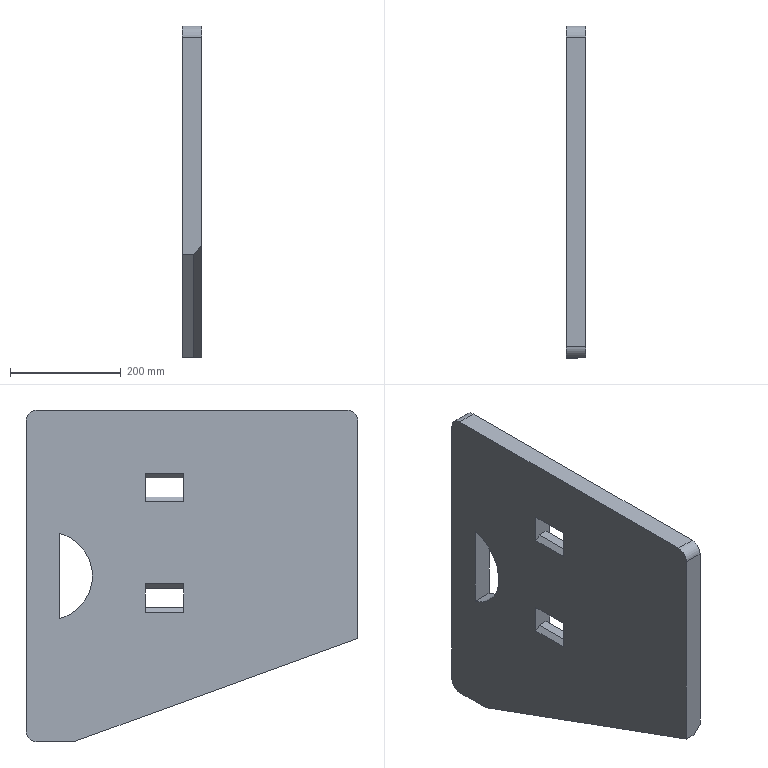Part | SolidWorks | features Chamfer 1, Extrusion 1, Fillet 1, ICE 1 | 1 solid | 29 faces | box 35 x 600 x 600 mm | volume 10412431 mm3 | plane 25 | cylinder 4 | commonest cylinder face diameters 40 x3 160 x1
STEP:
#1=CARTESIAN_POINT('',(17.5,15.,-366.));
#2=VERTEX_POINT('',#1);
#3=CARTESIAN_POINT('',(17.5,85.,-366.));
#4=VERTEX_POINT('',#3);
#5=CARTESIAN_POINT('',(17.5,15.,-366.));
#6=DIRECTION('',(0.,1.,0.));
#7=VECTOR('',#6,1000.);
#8=LINE('',#5,#7);
#9=EDGE_CURVE('',#2,#4,#8,.T.);
#10=ORIENTED_EDGE('',*,*,#9,.F.);
#11=CARTESIAN_POINT('',(17.5,15.,-314.));
#12=VERTEX_POINT('',#11);
#13=CARTESIAN_POINT('',(17.5,15.,-366.));
#14=DIRECTION('',(0.,0.,-1.));
#15=VECTOR('',#14,1000.);
#16=LINE('',#13,#15);
#17=EDGE_CURVE('',#12,#2,#16,.T.);
#18=ORIENTED_EDGE('',*,*,#17,.F.);
#19=CARTESIAN_POINT('',(17.5,85.,-314.));
#20=VERTEX_POINT('',#19);
#21=CARTESIAN_POINT('',(17.5,15.,-314.));
#22=DIRECTION('',(0.,1.,0.));
#23=VECTOR('',#22,1000.);
#24=LINE('',#21,#23);
#25=EDGE_CURVE('',#12,#20,#24,.T.);
#26=ORIENTED_EDGE('',*,*,#25,.T.);
#27=CARTESIAN_POINT('',(17.5,85.,-366.));
#28=DIRECTION('',(0.,0.,-1.));
#29=VECTOR('',#28,1000.);
#30=LINE('',#27,#29);
#31=EDGE_CURVE('',#20,#4,#30,.T.);
#32=ORIENTED_EDGE('',*,*,#31,.T.);
#33=EDGE_LOOP('',(#10,#18,#26,#32));
#34=FACE_BOUND('',#33,.T.);
#35=CARTESIAN_POINT('',(17.5,15.,-166.));
#36=VERTEX_POINT('',#35);
#37=CARTESIAN_POINT('',(17.5,85.,-166.));
#38=VERTEX_POINT('',#37);
#39=CARTESIAN_POINT('',(17.5,15.,-166.));
#40=DIRECTION('',(0.,1.,0.));
#41=VECTOR('',#40,1000.);
#42=LINE('',#39,#41);
#43=EDGE_CURVE('',#36,#38,#42,.T.);
#44=ORIENTED_EDGE('',*,*,#43,.F.);
#45=CARTESIAN_POINT('',(17.5,15.,-114.));
#46=VERTEX_POINT('',#45);
#47=CARTESIAN_POINT('',(17.5,15.,-114.));
#48=DIRECTION('',(0.,0.,-1.));
#49=VECTOR('',#48,1000.);
#50=LINE('',#47,#49);
#51=EDGE_CURVE('',#46,#36,#50,.T.);
#52=ORIENTED_EDGE('',*,*,#51,.F.);
#53=CARTESIAN_POINT('',(17.5,85.,-114.));
#54=VERTEX_POINT('',#53);
#55=CARTESIAN_POINT('',(17.5,15.,-114.));
#56=DIRECTION('',(0.,1.,0.));
#57=VECTOR('',#56,1000.);
#58=LINE('',#55,#57);
#59=EDGE_CURVE('',#46,#54,#58,.T.);
#60=ORIENTED_EDGE('',*,*,#59,.T.);
#61=CARTESIAN_POINT('',(17.5,85.,-114.));
#62=DIRECTION('',(0.,0.,-1.));
#63=VECTOR('',#62,1000.);
#64=LINE('',#61,#63);
#65=EDGE_CURVE('',#54,#38,#64,.T.);
#66=ORIENTED_EDGE('',*,*,#65,.T.);
#67=EDGE_LOOP('',(#44,#52,#60,#66));
#68=FACE_BOUND('',#67,.T.);
#69=CARTESIAN_POINT('',(17.5,-300.,-20.));
#70=VERTEX_POINT('',#69);
#71=CARTESIAN_POINT('',(17.5,-300.,-397.037));
#72=VERTEX_POINT('',#71);
#73=CARTESIAN_POINT('',(17.5,-300.,-413.));
#74=DIRECTION('',(0.,0.,-1.));
#75=VECTOR('',#74,1000.);
#76=LINE('',#73,#75);
#77=EDGE_CURVE('',#70,#72,#76,.T.);
#78=ORIENTED_EDGE('',*,*,#77,.T.);
#79=CARTESIAN_POINT('',(17.5,257.635,-600.));
#80=VERTEX_POINT('',#79);
#81=CARTESIAN_POINT('',(17.5,-162.699,-447.011));
#82=DIRECTION('',(0.,0.9397,-0.342));
#83=VECTOR('',#82,1000.);
#84=LINE('',#81,#83);
#85=EDGE_CURVE('',#72,#80,#84,.T.);
#86=ORIENTED_EDGE('',*,*,#85,.T.);
#87=CARTESIAN_POINT('',(17.5,280.,-600.));
#88=VERTEX_POINT('',#87);
#89=CARTESIAN_POINT('',(17.5,300.,-600.));
#90=DIRECTION('',(0.,1.,0.));
#91=VECTOR('',#90,1000.);
#92=LINE('',#89,#91);
#93=EDGE_CURVE('',#80,#88,#92,.T.);
#94=ORIENTED_EDGE('',*,*,#93,.T.);
#95=CARTESIAN_POINT('',(17.5,300.,-580.));
#96=VERTEX_POINT('',#95);
#97=CARTESIAN_POINT('',(17.5,280.,-580.));
#98=DIRECTION('',(1.,0.,0.));
#99=DIRECTION('',(0.,0.,1.));
#100=AXIS2_PLACEMENT_3D('',#97,#98,#99);
#101=CIRCLE('',#100,20.);
#102=EDGE_CURVE('',#88,#96,#101,.T.);
#103=ORIENTED_EDGE('',*,*,#102,.T.);
#104=CARTESIAN_POINT('',(17.5,300.,-20.));
#105=VERTEX_POINT('',#104);
#106=CARTESIAN_POINT('',(17.5,300.,0.));
#107=DIRECTION('',(0.,0.,1.));
#108=VECTOR('',#107,1000.);
#109=LINE('',#106,#108);
#110=EDGE_CURVE('',#96,#105,#109,.T.);
#111=ORIENTED_EDGE('',*,*,#110,.T.);
#112=CARTESIAN_POINT('',(17.5,280.,0.));
#113=VERTEX_POINT('',#112);
#114=CARTESIAN_POINT('',(17.5,280.,-20.));
#115=DIRECTION('',(1.,0.,0.));
#116=DIRECTION('',(0.,0.,1.));
#117=AXIS2_PLACEMENT_3D('',#114,#115,#116);
#118=CIRCLE('',#117,20.);
#119=EDGE_CURVE('',#105,#113,#118,.T.);
#120=ORIENTED_EDGE('',*,*,#119,.T.);
#121=CARTESIAN_POINT('',(17.5,-280.,0.));
#122=VERTEX_POINT('',#121);
#123=CARTESIAN_POINT('',(17.5,-300.,0.));
#124=DIRECTION('',(0.,-1.,0.));
#125=VECTOR('',#124,1000.);
#126=LINE('',#123,#125);
#127=EDGE_CURVE('',#113,#122,#126,.T.);
#128=ORIENTED_EDGE('',*,*,#127,.T.);
#129=CARTESIAN_POINT('',(17.5,-280.,-20.));
#130=DIRECTION('',(1.,0.,0.));
#131=DIRECTION('',(0.,0.,1.));
#132=AXIS2_PLACEMENT_3D('',#129,#130,#131);
#133=CIRCLE('',#132,20.);
#134=EDGE_CURVE('',#122,#70,#133,.T.);
#135=ORIENTED_EDGE('',*,*,#134,.T.);
#136=EDGE_LOOP('',(#78,#86,#94,#103,#111,#120,#128,#135));
#137=FACE_OUTER_BOUND('',#136,.T.);
#138=CARTESIAN_POINT('',(17.5,240.,-222.54));
#139=VERTEX_POINT('',#138);
#140=CARTESIAN_POINT('',(17.5,240.,-377.46));
#141=VERTEX_POINT('',#140);
#142=CARTESIAN_POINT('',(17.5,260.,-300.));
#143=DIRECTION('',(1.,0.,0.));
#144=DIRECTION('',(0.,0.,-1.));
#145=AXIS2_PLACEMENT_3D('',#142,#143,#144);
#146=CIRCLE('',#145,80.);
#147=EDGE_CURVE('',#139,#141,#146,.T.);
#148=ORIENTED_EDGE('',*,*,#147,.F.);
#149=CARTESIAN_POINT('',(17.5,240.,-222.54));
#150=DIRECTION('',(0.,0.,1.));
#151=VECTOR('',#150,1000.);
#152=LINE('',#149,#151);
#153=EDGE_CURVE('',#141,#139,#152,.T.);
#154=ORIENTED_EDGE('',*,*,#153,.F.);
#155=EDGE_LOOP('',(#148,#154));
#156=FACE_BOUND('',#155,.T.);
#157=CARTESIAN_POINT('',(17.5,0.,0.));
#158=DIRECTION('',(-1.,0.,0.));
#159=DIRECTION('',(0.,0.,1.));
#160=AXIS2_PLACEMENT_3D('',#157,#158,#159);
#161=PLANE('',#160);
#162=ADVANCED_FACE('',(#34,#68,#137,#156),#161,.F.);
#163=CARTESIAN_POINT('',(-17.5,15.,-366.));
#164=VERTEX_POINT('',#163);
#165=CARTESIAN_POINT('',(-17.5,15.,-314.));
#166=VERTEX_POINT('',#165);
#167=CARTESIAN_POINT('',(-17.5,15.,-366.));
#168=DIRECTION('',(0.,0.,1.));
#169=VECTOR('',#168,1000.);
#170=LINE('',#167,#169);
#171=EDGE_CURVE('',#164,#166,#170,.T.);
#172=ORIENTED_EDGE('',*,*,#171,.F.);
#173=CARTESIAN_POINT('',(-17.5,85.,-366.));
#174=VERTEX_POINT('',#173);
#175=CARTESIAN_POINT('',(-17.5,15.,-366.));
#176=DIRECTION('',(0.,1.,0.));
#177=VECTOR('',#176,1000.);
#178=LINE('',#175,#177);
#179=EDGE_CURVE('',#164,#174,#178,.T.);
#180=ORIENTED_EDGE('',*,*,#179,.T.);
#181=CARTESIAN_POINT('',(-17.5,85.,-314.));
#182=VERTEX_POINT('',#181);
#183=CARTESIAN_POINT('',(-17.5,85.,-366.));
#184=DIRECTION('',(0.,0.,1.));
#185=VECTOR('',#184,1000.);
#186=LINE('',#183,#185);
#187=EDGE_CURVE('',#174,#182,#186,.T.);
#188=ORIENTED_EDGE('',*,*,#187,.T.);
#189=CARTESIAN_POINT('',(-17.5,15.,-314.));
#190=DIRECTION('',(0.,1.,0.));
#191=VECTOR('',#190,1000.);
#192=LINE('',#189,#191);
#193=EDGE_CURVE('',#166,#182,#192,.T.);
#194=ORIENTED_EDGE('',*,*,#193,.F.);
#195=EDGE_LOOP('',(#172,#180,#188,#194));
#196=FACE_BOUND('',#195,.T.);
#197=CARTESIAN_POINT('',(-17.5,15.,-166.));
#198=VERTEX_POINT('',#197);
#199=CARTESIAN_POINT('',(-17.5,15.,-114.));
#200=VERTEX_POINT('',#199);
#201=CARTESIAN_POINT('',(-17.5,15.,-114.));
#202=DIRECTION('',(0.,0.,1.));
#203=VECTOR('',#202,1000.);
#204=LINE('',#201,#203);
#205=EDGE_CURVE('',#198,#200,#204,.T.);
#206=ORIENTED_EDGE('',*,*,#205,.F.);
#207=CARTESIAN_POINT('',(-17.5,85.,-166.));
#208=VERTEX_POINT('',#207);
#209=CARTESIAN_POINT('',(-17.5,15.,-166.));
#210=DIRECTION('',(0.,1.,0.));
#211=VECTOR('',#210,1000.);
#212=LINE('',#209,#211);
#213=EDGE_CURVE('',#198,#208,#212,.T.);
#214=ORIENTED_EDGE('',*,*,#213,.T.);
#215=CARTESIAN_POINT('',(-17.5,85.,-114.));
#216=VERTEX_POINT('',#215);
#217=CARTESIAN_POINT('',(-17.5,85.,-114.));
#218=DIRECTION('',(0.,0.,1.));
#219=VECTOR('',#218,1000.);
#220=LINE('',#217,#219);
#221=EDGE_CURVE('',#208,#216,#220,.T.);
#222=ORIENTED_EDGE('',*,*,#221,.T.);
#223=CARTESIAN_POINT('',(-17.5,15.,-114.));
#224=DIRECTION('',(0.,1.,0.));
#225=VECTOR('',#224,1000.);
#226=LINE('',#223,#225);
#227=EDGE_CURVE('',#200,#216,#226,.T.);
#228=ORIENTED_EDGE('',*,*,#227,.F.);
#229=EDGE_LOOP('',(#206,#214,#222,#228));
#230=FACE_BOUND('',#229,.T.);
#231=CARTESIAN_POINT('',(-17.5,300.,-580.));
#232=VERTEX_POINT('',#231);
#233=CARTESIAN_POINT('',(-17.5,300.,-20.));
#234=VERTEX_POINT('',#233);
#235=CARTESIAN_POINT('',(-17.5,300.,0.));
#236=DIRECTION('',(0.,0.,1.));
#237=VECTOR('',#236,1000.);
#238=LINE('',#235,#237);
#239=EDGE_CURVE('',#232,#234,#238,.T.);
#240=ORIENTED_EDGE('',*,*,#239,.F.);
#241=CARTESIAN_POINT('',(-17.5,280.,-600.));
#242=VERTEX_POINT('',#241);
#243=CARTESIAN_POINT('',(-17.5,280.,-580.));
#244=DIRECTION('',(-1.,0.,0.));
#245=DIRECTION('',(0.,0.,1.));
#246=AXIS2_PLACEMENT_3D('',#243,#244,#245);
#247=CIRCLE('',#246,20.);
#248=EDGE_CURVE('',#232,#242,#247,.T.);
#249=ORIENTED_EDGE('',*,*,#248,.T.);
#250=CARTESIAN_POINT('',(-17.5,213.778,-600.));
#251=VERTEX_POINT('',#250);
#252=CARTESIAN_POINT('',(-17.5,300.,-600.));
#253=DIRECTION('',(0.,1.,0.));
#254=VECTOR('',#253,1000.);
#255=LINE('',#252,#254);
#256=EDGE_CURVE('',#251,#242,#255,.T.);
#257=ORIENTED_EDGE('',*,*,#256,.F.);
#258=CARTESIAN_POINT('',(-17.5,-300.,-413.));
#259=VERTEX_POINT('',#258);
#260=CARTESIAN_POINT('',(-17.5,213.778,-600.));
#261=DIRECTION('',(0.,0.9397,-0.342));
#262=VECTOR('',#261,1000.);
#263=LINE('',#260,#262);
#264=EDGE_CURVE('',#259,#251,#263,.T.);
#265=ORIENTED_EDGE('',*,*,#264,.F.);
#266=CARTESIAN_POINT('',(-17.5,-300.,-20.));
#267=VERTEX_POINT('',#266);
#268=CARTESIAN_POINT('',(-17.5,-300.,-413.));
#269=DIRECTION('',(0.,0.,-1.));
#270=VECTOR('',#269,1000.);
#271=LINE('',#268,#270);
#272=EDGE_CURVE('',#267,#259,#271,.T.);
#273=ORIENTED_EDGE('',*,*,#272,.F.);
#274=CARTESIAN_POINT('',(-17.5,-280.,0.));
#275=VERTEX_POINT('',#274);
#276=CARTESIAN_POINT('',(-17.5,-280.,-20.));
#277=DIRECTION('',(-1.,0.,0.));
#278=DIRECTION('',(0.,0.,1.));
#279=AXIS2_PLACEMENT_3D('',#276,#277,#278);
#280=CIRCLE('',#279,20.);
#281=EDGE_CURVE('',#267,#275,#280,.T.);
#282=ORIENTED_EDGE('',*,*,#281,.T.);
#283=CARTESIAN_POINT('',(-17.5,280.,0.));
#284=VERTEX_POINT('',#283);
#285=CARTESIAN_POINT('',(-17.5,0.,0.));
#286=DIRECTION('',(0.,-1.,0.));
#287=VECTOR('',#286,1000.);
#288=LINE('',#285,#287);
#289=EDGE_CURVE('',#284,#275,#288,.T.);
#290=ORIENTED_EDGE('',*,*,#289,.F.);
#291=CARTESIAN_POINT('',(-17.5,280.,-20.));
#292=DIRECTION('',(-1.,0.,0.));
#293=DIRECTION('',(0.,0.,1.));
#294=AXIS2_PLACEMENT_3D('',#291,#292,#293);
#295=CIRCLE('',#294,20.);
#296=EDGE_CURVE('',#284,#234,#295,.T.);
#297=ORIENTED_EDGE('',*,*,#296,.T.);
#298=EDGE_LOOP('',(#240,#249,#257,#265,#273,#282,#290,#297));
#299=FACE_OUTER_BOUND('',#298,.T.);
#300=CARTESIAN_POINT('',(-17.5,240.,-377.46));
#301=VERTEX_POINT('',#300);
#302=CARTESIAN_POINT('',(-17.5,240.,-222.54));
#303=VERTEX_POINT('',#302);
#304=CARTESIAN_POINT('',(-17.5,240.,-222.54));
#305=DIRECTION('',(0.,0.,1.));
#306=VECTOR('',#305,1000.);
#307=LINE('',#304,#306);
#308=EDGE_CURVE('',#301,#303,#307,.T.);
#309=ORIENTED_EDGE('',*,*,#308,.T.);
#310=CARTESIAN_POINT('',(-17.5,260.,-300.));
#311=DIRECTION('',(1.,0.,0.));
#312=DIRECTION('',(0.,0.,-1.));
#313=AXIS2_PLACEMENT_3D('',#310,#311,#312);
#314=CIRCLE('',#313,80.);
#315=EDGE_CURVE('',#303,#301,#314,.T.);
#316=ORIENTED_EDGE('',*,*,#315,.T.);
#317=EDGE_LOOP('',(#309,#316));
#318=FACE_BOUND('',#317,.T.);
#319=CARTESIAN_POINT('',(-17.5,0.,0.));
#320=DIRECTION('',(-1.,0.,0.));
#321=DIRECTION('',(0.,0.,1.));
#322=AXIS2_PLACEMENT_3D('',#319,#320,#321);
#323=PLANE('',#322);
#324=ADVANCED_FACE('',(#196,#230,#299,#318),#323,.T.);
#325=CARTESIAN_POINT('',(2.5,-300.,-413.));
#326=VERTEX_POINT('',#325);
#327=CARTESIAN_POINT('',(17.5,-300.,-413.));
#328=DIRECTION('',(-1.,0.,0.));
#329=VECTOR('',#328,1000.);
#330=LINE('',#327,#329);
#331=EDGE_CURVE('',#326,#259,#330,.T.);
#332=ORIENTED_EDGE('',*,*,#331,.F.);
#333=CARTESIAN_POINT('',(-7.439,-300.,-423.576));
#334=DIRECTION('',(0.6848,0.,0.7287));
#335=VECTOR('',#334,1000.);
#336=LINE('',#333,#335);
#337=EDGE_CURVE('',#326,#72,#336,.T.);
#338=ORIENTED_EDGE('',*,*,#337,.T.);
#339=ORIENTED_EDGE('',*,*,#77,.F.);
#340=CARTESIAN_POINT('',(17.5,-300.,-20.));
#341=DIRECTION('',(-1.,0.,0.));
#342=VECTOR('',#341,1000.);
#343=LINE('',#340,#342);
#344=EDGE_CURVE('',#70,#267,#343,.T.);
#345=ORIENTED_EDGE('',*,*,#344,.T.);
#346=ORIENTED_EDGE('',*,*,#272,.T.);
#347=EDGE_LOOP('',(#332,#338,#339,#345,#346));
#348=FACE_OUTER_BOUND('',#347,.T.);
#349=CARTESIAN_POINT('',(17.5,-300.,-413.));
#350=DIRECTION('',(0.,1.,0.));
#351=DIRECTION('',(0.,0.,1.));
#352=AXIS2_PLACEMENT_3D('',#349,#350,#351);
#353=PLANE('',#352);
#354=ADVANCED_FACE('',(#348),#353,.F.);
#355=CARTESIAN_POINT('',(2.5,213.778,-600.));
#356=VERTEX_POINT('',#355);
#357=CARTESIAN_POINT('',(17.5,213.778,-600.));
#358=DIRECTION('',(-1.,0.,0.));
#359=VECTOR('',#358,1000.);
#360=LINE('',#357,#359);
#361=EDGE_CURVE('',#356,#251,#360,.T.);
#362=ORIENTED_EDGE('',*,*,#361,.F.);
#363=CARTESIAN_POINT('',(2.5,213.778,-600.));
#364=DIRECTION('',(0.,-0.9397,0.342));
#365=VECTOR('',#364,1000.);
#366=LINE('',#363,#365);
#367=EDGE_CURVE('',#356,#326,#366,.T.);
#368=ORIENTED_EDGE('',*,*,#367,.T.);
#369=ORIENTED_EDGE('',*,*,#331,.T.);
#370=ORIENTED_EDGE('',*,*,#264,.T.);
#371=EDGE_LOOP('',(#362,#368,#369,#370));
#372=FACE_OUTER_BOUND('',#371,.T.);
#373=CARTESIAN_POINT('',(17.5,213.778,-600.));
#374=DIRECTION('',(0.,0.342,0.9397));
#375=DIRECTION('',(0.,-0.9397,0.342));
#376=AXIS2_PLACEMENT_3D('',#373,#374,#375);
#377=PLANE('',#376);
#378=ADVANCED_FACE('',(#372),#377,.F.);
#379=ORIENTED_EDGE('',*,*,#93,.F.);
#380=CARTESIAN_POINT('',(-111.207,-118.678,-600.));
#381=DIRECTION('',(-0.3236,-0.9462,0.));
#382=VECTOR('',#381,1000.);
#383=LINE('',#380,#382);
#384=EDGE_CURVE('',#80,#356,#383,.T.);
#385=ORIENTED_EDGE('',*,*,#384,.T.);
#386=ORIENTED_EDGE('',*,*,#361,.T.);
#387=ORIENTED_EDGE('',*,*,#256,.T.);
#388=CARTESIAN_POINT('',(17.5,280.,-600.));
#389=DIRECTION('',(1.,0.,0.));
#390=VECTOR('',#389,1000.);
#391=LINE('',#388,#390);
#392=EDGE_CURVE('',#242,#88,#391,.T.);
#393=ORIENTED_EDGE('',*,*,#392,.T.);
#394=EDGE_LOOP('',(#379,#385,#386,#387,#393));
#395=FACE_OUTER_BOUND('',#394,.T.);
#396=CARTESIAN_POINT('',(17.5,300.,-600.));
#397=DIRECTION('',(0.,0.,1.));
#398=DIRECTION('',(1.,0.,0.));
#399=AXIS2_PLACEMENT_3D('',#396,#397,#398);
#400=PLANE('',#399);
#401=ADVANCED_FACE('',(#395),#400,.F.);
#402=ORIENTED_EDGE('',*,*,#110,.F.);
#403=CARTESIAN_POINT('',(17.5,300.,-580.));
#404=DIRECTION('',(-1.,0.,0.));
#405=VECTOR('',#404,1000.);
#406=LINE('',#403,#405);
#407=EDGE_CURVE('',#96,#232,#406,.T.);
#408=ORIENTED_EDGE('',*,*,#407,.T.);
#409=ORIENTED_EDGE('',*,*,#239,.T.);
#410=CARTESIAN_POINT('',(17.5,300.,-20.));
#411=DIRECTION('',(1.,0.,0.));
#412=VECTOR('',#411,1000.);
#413=LINE('',#410,#412);
#414=EDGE_CURVE('',#234,#105,#413,.T.);
#415=ORIENTED_EDGE('',*,*,#414,.T.);
#416=EDGE_LOOP('',(#402,#408,#409,#415));
#417=FACE_OUTER_BOUND('',#416,.T.);
#418=CARTESIAN_POINT('',(17.5,300.,0.));
#419=DIRECTION('',(0.,-1.,0.));
#420=DIRECTION('',(0.,0.,-1.));
#421=AXIS2_PLACEMENT_3D('',#418,#419,#420);
#422=PLANE('',#421);
#423=ADVANCED_FACE('',(#417),#422,.F.);
#424=ORIENTED_EDGE('',*,*,#289,.T.);
#425=CARTESIAN_POINT('',(17.5,-280.,0.));
#426=DIRECTION('',(1.,0.,0.));
#427=VECTOR('',#426,1000.);
#428=LINE('',#425,#427);
#429=EDGE_CURVE('',#275,#122,#428,.T.);
#430=ORIENTED_EDGE('',*,*,#429,.T.);
#431=ORIENTED_EDGE('',*,*,#127,.F.);
#432=CARTESIAN_POINT('',(17.5,280.,0.));
#433=DIRECTION('',(-1.,0.,0.));
#434=VECTOR('',#433,1000.);
#435=LINE('',#432,#434);
#436=EDGE_CURVE('',#113,#284,#435,.T.);
#437=ORIENTED_EDGE('',*,*,#436,.T.);
#438=EDGE_LOOP('',(#424,#430,#431,#437));
#439=FACE_OUTER_BOUND('',#438,.T.);
#440=CARTESIAN_POINT('',(17.5,0.,0.));
#441=DIRECTION('',(0.,0.,-1.));
#442=DIRECTION('',(-1.,0.,0.));
#443=AXIS2_PLACEMENT_3D('',#440,#441,#442);
#444=PLANE('',#443);
#445=ADVANCED_FACE('',(#439),#444,.F.);
#446=ORIENTED_EDGE('',*,*,#315,.F.);
#447=CARTESIAN_POINT('',(17.5,240.,-222.54));
#448=DIRECTION('',(-1.,0.,0.));
#449=VECTOR('',#448,1000.);
#450=LINE('',#447,#449);
#451=EDGE_CURVE('',#139,#303,#450,.T.);
#452=ORIENTED_EDGE('',*,*,#451,.F.);
#453=ORIENTED_EDGE('',*,*,#147,.T.);
#454=CARTESIAN_POINT('',(17.5,240.,-377.46));
#455=DIRECTION('',(-1.,0.,0.));
#456=VECTOR('',#455,1000.);
#457=LINE('',#454,#456);
#458=EDGE_CURVE('',#141,#301,#457,.T.);
#459=ORIENTED_EDGE('',*,*,#458,.T.);
#460=EDGE_LOOP('',(#446,#452,#453,#459));
#461=FACE_OUTER_BOUND('',#460,.T.);
#462=CARTESIAN_POINT('',(17.5,260.,-300.));
#463=DIRECTION('',(-1.,0.,0.));
#464=DIRECTION('',(0.,0.,1.));
#465=AXIS2_PLACEMENT_3D('',#462,#463,#464);
#466=CYLINDRICAL_SURFACE('',#465,80.);
#467=ADVANCED_FACE('',(#461),#466,.F.);
#468=ORIENTED_EDGE('',*,*,#308,.F.);
#469=ORIENTED_EDGE('',*,*,#458,.F.);
#470=ORIENTED_EDGE('',*,*,#153,.T.);
#471=ORIENTED_EDGE('',*,*,#451,.T.);
#472=EDGE_LOOP('',(#468,#469,#470,#471));
#473=FACE_OUTER_BOUND('',#472,.T.);
#474=CARTESIAN_POINT('',(17.5,240.,-222.54));
#475=DIRECTION('',(0.,-1.,0.));
#476=DIRECTION('',(0.,0.,-1.));
#477=AXIS2_PLACEMENT_3D('',#474,#475,#476);
#478=PLANE('',#477);
#479=ADVANCED_FACE('',(#473),#478,.T.);
#480=CARTESIAN_POINT('',(-8.5,85.,-157.5));
#481=VERTEX_POINT('',#480);
#482=CARTESIAN_POINT('',(-17.5,85.,-166.));
#483=DIRECTION('',(-0.727,0.,-0.6866));
#484=VECTOR('',#483,1000.);
#485=LINE('',#482,#484);
#486=EDGE_CURVE('',#481,#208,#485,.T.);
#487=ORIENTED_EDGE('',*,*,#486,.T.);
#488=ORIENTED_EDGE('',*,*,#213,.F.);
#489=CARTESIAN_POINT('',(-8.5,15.,-157.5));
#490=VERTEX_POINT('',#489);
#491=CARTESIAN_POINT('',(-17.5,15.,-166.));
#492=DIRECTION('',(-0.727,0.,-0.6866));
#493=VECTOR('',#492,1000.);
#494=LINE('',#491,#493);
#495=EDGE_CURVE('',#490,#198,#494,.T.);
#496=ORIENTED_EDGE('',*,*,#495,.F.);
#497=CARTESIAN_POINT('',(-8.5,15.,-157.5));
#498=DIRECTION('',(0.,1.,0.));
#499=VECTOR('',#498,1000.);
#500=LINE('',#497,#499);
#501=EDGE_CURVE('',#490,#481,#500,.T.);
#502=ORIENTED_EDGE('',*,*,#501,.T.);
#503=EDGE_LOOP('',(#487,#488,#496,#502));
#504=FACE_OUTER_BOUND('',#503,.T.);
#505=CARTESIAN_POINT('',(-17.5,15.,-166.));
#506=DIRECTION('',(0.6866,0.,-0.727));
#507=DIRECTION('',(-0.727,0.,-0.6866));
#508=AXIS2_PLACEMENT_3D('',#505,#506,#507);
#509=PLANE('',#508);
#510=ADVANCED_FACE('',(#504),#509,.F.);
#511=CARTESIAN_POINT('',(8.5,85.,-157.5));
#512=VERTEX_POINT('',#511);
#513=CARTESIAN_POINT('',(-8.5,85.,-157.5));
#514=DIRECTION('',(-1.,0.,0.));
#515=VECTOR('',#514,1000.);
#516=LINE('',#513,#515);
#517=EDGE_CURVE('',#512,#481,#516,.T.);
#518=ORIENTED_EDGE('',*,*,#517,.T.);
#519=ORIENTED_EDGE('',*,*,#501,.F.);
#520=CARTESIAN_POINT('',(8.5,15.,-157.5));
#521=VERTEX_POINT('',#520);
#522=CARTESIAN_POINT('',(-8.5,15.,-157.5));
#523=DIRECTION('',(-1.,0.,0.));
#524=VECTOR('',#523,1000.);
#525=LINE('',#522,#524);
#526=EDGE_CURVE('',#521,#490,#525,.T.);
#527=ORIENTED_EDGE('',*,*,#526,.F.);
#528=CARTESIAN_POINT('',(8.5,15.,-157.5));
#529=DIRECTION('',(0.,1.,0.));
#530=VECTOR('',#529,1000.);
#531=LINE('',#528,#530);
#532=EDGE_CURVE('',#521,#512,#531,.T.);
#533=ORIENTED_EDGE('',*,*,#532,.T.);
#534=EDGE_LOOP('',(#518,#519,#527,#533));
#535=FACE_OUTER_BOUND('',#534,.T.);
#536=CARTESIAN_POINT('',(-8.5,15.,-157.5));
#537=DIRECTION('',(0.,0.,-1.));
#538=DIRECTION('',(-1.,0.,0.));
#539=AXIS2_PLACEMENT_3D('',#536,#537,#538);
#540=PLANE('',#539);
#541=ADVANCED_FACE('',(#535),#540,.F.);
#542=CARTESIAN_POINT('',(8.5,85.,-157.5));
#543=DIRECTION('',(-0.727,0.,0.6866));
#544=VECTOR('',#543,1000.);
#545=LINE('',#542,#544);
#546=EDGE_CURVE('',#38,#512,#545,.T.);
#547=ORIENTED_EDGE('',*,*,#546,.T.);
#548=ORIENTED_EDGE('',*,*,#532,.F.);
#549=CARTESIAN_POINT('',(8.5,15.,-157.5));
#550=DIRECTION('',(-0.727,0.,0.6866));
#551=VECTOR('',#550,1000.);
#552=LINE('',#549,#551);
#553=EDGE_CURVE('',#36,#521,#552,.T.);
#554=ORIENTED_EDGE('',*,*,#553,.F.);
#555=ORIENTED_EDGE('',*,*,#43,.T.);
#556=EDGE_LOOP('',(#547,#548,#554,#555));
#557=FACE_OUTER_BOUND('',#556,.T.);
#558=CARTESIAN_POINT('',(8.5,15.,-157.5));
#559=DIRECTION('',(-0.6866,0.,-0.727));
#560=DIRECTION('',(-0.727,0.,0.6866));
#561=AXIS2_PLACEMENT_3D('',#558,#559,#560);
#562=PLANE('',#561);
#563=ADVANCED_FACE('',(#557),#562,.F.);
#564=CARTESIAN_POINT('',(8.5,85.,-122.5));
#565=VERTEX_POINT('',#564);
#566=CARTESIAN_POINT('',(8.5,85.,-122.5));
#567=DIRECTION('',(0.727,0.,0.6866));
#568=VECTOR('',#567,1000.);
#569=LINE('',#566,#568);
#570=EDGE_CURVE('',#565,#54,#569,.T.);
#571=ORIENTED_EDGE('',*,*,#570,.T.);
#572=ORIENTED_EDGE('',*,*,#59,.F.);
#573=CARTESIAN_POINT('',(8.5,15.,-122.5));
#574=VERTEX_POINT('',#573);
#575=CARTESIAN_POINT('',(8.5,15.,-122.5));
#576=DIRECTION('',(0.727,0.,0.6866));
#577=VECTOR('',#576,1000.);
#578=LINE('',#575,#577);
#579=EDGE_CURVE('',#574,#46,#578,.T.);
#580=ORIENTED_EDGE('',*,*,#579,.F.);
#581=CARTESIAN_POINT('',(8.5,15.,-122.5));
#582=DIRECTION('',(0.,1.,0.));
#583=VECTOR('',#582,1000.);
#584=LINE('',#581,#583);
#585=EDGE_CURVE('',#574,#565,#584,.T.);
#586=ORIENTED_EDGE('',*,*,#585,.T.);
#587=EDGE_LOOP('',(#571,#572,#580,#586));
#588=FACE_OUTER_BOUND('',#587,.T.);
#589=CARTESIAN_POINT('',(8.5,15.,-122.5));
#590=DIRECTION('',(-0.6866,0.,0.727));
#591=DIRECTION('',(0.727,0.,0.6866));
#592=AXIS2_PLACEMENT_3D('',#589,#590,#591);
#593=PLANE('',#592);
#594=ADVANCED_FACE('',(#588),#593,.F.);
#595=CARTESIAN_POINT('',(-8.5,85.,-122.5));
#596=VERTEX_POINT('',#595);
#597=CARTESIAN_POINT('',(-8.5,85.,-122.5));
#598=DIRECTION('',(1.,0.,0.));
#599=VECTOR('',#598,1000.);
#600=LINE('',#597,#599);
#601=EDGE_CURVE('',#596,#565,#600,.T.);
#602=ORIENTED_EDGE('',*,*,#601,.T.);
#603=ORIENTED_EDGE('',*,*,#585,.F.);
#604=CARTESIAN_POINT('',(-8.5,15.,-122.5));
#605=VERTEX_POINT('',#604);
#606=CARTESIAN_POINT('',(-8.5,15.,-122.5));
#607=DIRECTION('',(1.,0.,0.));
#608=VECTOR('',#607,1000.);
#609=LINE('',#606,#608);
#610=EDGE_CURVE('',#605,#574,#609,.T.);
#611=ORIENTED_EDGE('',*,*,#610,.F.);
#612=CARTESIAN_POINT('',(-8.5,15.,-122.5));
#613=DIRECTION('',(0.,1.,0.));
#614=VECTOR('',#613,1000.);
#615=LINE('',#612,#614);
#616=EDGE_CURVE('',#605,#596,#615,.T.);
#617=ORIENTED_EDGE('',*,*,#616,.T.);
#618=EDGE_LOOP('',(#602,#603,#611,#617));
#619=FACE_OUTER_BOUND('',#618,.T.);
#620=CARTESIAN_POINT('',(-8.5,15.,-122.5));
#621=DIRECTION('',(0.,0.,1.));
#622=DIRECTION('',(1.,0.,0.));
#623=AXIS2_PLACEMENT_3D('',#620,#621,#622);
#624=PLANE('',#623);
#625=ADVANCED_FACE('',(#619),#624,.F.);
#626=CARTESIAN_POINT('',(-17.5,85.,-114.));
#627=DIRECTION('',(0.727,0.,-0.6866));
#628=VECTOR('',#627,1000.);
#629=LINE('',#626,#628);
#630=EDGE_CURVE('',#216,#596,#629,.T.);
#631=ORIENTED_EDGE('',*,*,#630,.T.);
#632=ORIENTED_EDGE('',*,*,#616,.F.);
#633=CARTESIAN_POINT('',(-17.5,15.,-114.));
#634=DIRECTION('',(0.727,0.,-0.6866));
#635=VECTOR('',#634,1000.);
#636=LINE('',#633,#635);
#637=EDGE_CURVE('',#200,#605,#636,.T.);
#638=ORIENTED_EDGE('',*,*,#637,.F.);
#639=ORIENTED_EDGE('',*,*,#227,.T.);
#640=EDGE_LOOP('',(#631,#632,#638,#639));
#641=FACE_OUTER_BOUND('',#640,.T.);
#642=CARTESIAN_POINT('',(-17.5,15.,-114.));
#643=DIRECTION('',(0.6866,0.,0.727));
#644=DIRECTION('',(0.727,0.,-0.6866));
#645=AXIS2_PLACEMENT_3D('',#642,#643,#644);
#646=PLANE('',#645);
#647=ADVANCED_FACE('',(#641),#646,.F.);
#648=ORIENTED_EDGE('',*,*,#205,.T.);
#649=ORIENTED_EDGE('',*,*,#637,.T.);
#650=ORIENTED_EDGE('',*,*,#610,.T.);
#651=ORIENTED_EDGE('',*,*,#579,.T.);
#652=ORIENTED_EDGE('',*,*,#51,.T.);
#653=ORIENTED_EDGE('',*,*,#553,.T.);
#654=ORIENTED_EDGE('',*,*,#526,.T.);
#655=ORIENTED_EDGE('',*,*,#495,.T.);
#656=EDGE_LOOP('',(#648,#649,#650,#651,#652,#653,#654,#655));
#657=FACE_OUTER_BOUND('',#656,.T.);
#658=CARTESIAN_POINT('',(0.,15.,0.));
#659=DIRECTION('',(0.,-1.,0.));
#660=DIRECTION('',(0.,0.,-1.));
#661=AXIS2_PLACEMENT_3D('',#658,#659,#660);
#662=PLANE('',#661);
#663=ADVANCED_FACE('',(#657),#662,.F.);
#664=ORIENTED_EDGE('',*,*,#221,.F.);
#665=ORIENTED_EDGE('',*,*,#486,.F.);
#666=ORIENTED_EDGE('',*,*,#517,.F.);
#667=ORIENTED_EDGE('',*,*,#546,.F.);
#668=ORIENTED_EDGE('',*,*,#65,.F.);
#669=ORIENTED_EDGE('',*,*,#570,.F.);
#670=ORIENTED_EDGE('',*,*,#601,.F.);
#671=ORIENTED_EDGE('',*,*,#630,.F.);
#672=EDGE_LOOP('',(#664,#665,#666,#667,#668,#669,#670,#671));
#673=FACE_OUTER_BOUND('',#672,.T.);
#674=CARTESIAN_POINT('',(0.,85.,0.));
#675=DIRECTION('',(0.,-1.,0.));
#676=DIRECTION('',(0.,0.,-1.));
#677=AXIS2_PLACEMENT_3D('',#674,#675,#676);
#678=PLANE('',#677);
#679=ADVANCED_FACE('',(#673),#678,.T.);
#680=CARTESIAN_POINT('',(8.5,85.,-357.5));
#681=VERTEX_POINT('',#680);
#682=CARTESIAN_POINT('',(-8.5,85.,-357.5));
#683=VERTEX_POINT('',#682);
#684=CARTESIAN_POINT('',(-8.5,85.,-357.5));
#685=DIRECTION('',(-1.,0.,0.));
#686=VECTOR('',#685,1000.);
#687=LINE('',#684,#686);
#688=EDGE_CURVE('',#681,#683,#687,.T.);
#689=ORIENTED_EDGE('',*,*,#688,.T.);
#690=CARTESIAN_POINT('',(-8.5,15.,-357.5));
#691=VERTEX_POINT('',#690);
#692=CARTESIAN_POINT('',(-8.5,15.,-357.5));
#693=DIRECTION('',(0.,1.,0.));
#694=VECTOR('',#693,1000.);
#695=LINE('',#692,#694);
#696=EDGE_CURVE('',#691,#683,#695,.T.);
#697=ORIENTED_EDGE('',*,*,#696,.F.);
#698=CARTESIAN_POINT('',(8.5,15.,-357.5));
#699=VERTEX_POINT('',#698);
#700=CARTESIAN_POINT('',(-8.5,15.,-357.5));
#701=DIRECTION('',(-1.,0.,0.));
#702=VECTOR('',#701,1000.);
#703=LINE('',#700,#702);
#704=EDGE_CURVE('',#699,#691,#703,.T.);
#705=ORIENTED_EDGE('',*,*,#704,.F.);
#706=CARTESIAN_POINT('',(8.5,15.,-357.5));
#707=DIRECTION('',(0.,1.,0.));
#708=VECTOR('',#707,1000.);
#709=LINE('',#706,#708);
#710=EDGE_CURVE('',#699,#681,#709,.T.);
#711=ORIENTED_EDGE('',*,*,#710,.T.);
#712=EDGE_LOOP('',(#689,#697,#705,#711));
#713=FACE_OUTER_BOUND('',#712,.T.);
#714=CARTESIAN_POINT('',(-8.5,15.,-357.5));
#715=DIRECTION('',(0.,0.,-1.));
#716=DIRECTION('',(-1.,0.,0.));
#717=AXIS2_PLACEMENT_3D('',#714,#715,#716);
#718=PLANE('',#717);
#719=ADVANCED_FACE('',(#713),#718,.F.);
#720=CARTESIAN_POINT('',(8.5,85.,-357.5));
#721=DIRECTION('',(-0.727,0.,0.6866));
#722=VECTOR('',#721,1000.);
#723=LINE('',#720,#722);
#724=EDGE_CURVE('',#4,#681,#723,.T.);
#725=ORIENTED_EDGE('',*,*,#724,.T.);
#726=ORIENTED_EDGE('',*,*,#710,.F.);
#727=CARTESIAN_POINT('',(8.5,15.,-357.5));
#728=DIRECTION('',(-0.727,0.,0.6866));
#729=VECTOR('',#728,1000.);
#730=LINE('',#727,#729);
#731=EDGE_CURVE('',#2,#699,#730,.T.);
#732=ORIENTED_EDGE('',*,*,#731,.F.);
#733=ORIENTED_EDGE('',*,*,#9,.T.);
#734=EDGE_LOOP('',(#725,#726,#732,#733));
#735=FACE_OUTER_BOUND('',#734,.T.);
#736=CARTESIAN_POINT('',(8.5,15.,-357.5));
#737=DIRECTION('',(-0.6866,0.,-0.727));
#738=DIRECTION('',(-0.727,0.,0.6866));
#739=AXIS2_PLACEMENT_3D('',#736,#737,#738);
#740=PLANE('',#739);
#741=ADVANCED_FACE('',(#735),#740,.F.);
#742=CARTESIAN_POINT('',(8.5,85.,-322.5));
#743=VERTEX_POINT('',#742);
#744=CARTESIAN_POINT('',(8.5,85.,-322.5));
#745=DIRECTION('',(0.727,0.,0.6866));
#746=VECTOR('',#745,1000.);
#747=LINE('',#744,#746);
#748=EDGE_CURVE('',#743,#20,#747,.T.);
#749=ORIENTED_EDGE('',*,*,#748,.T.);
#750=ORIENTED_EDGE('',*,*,#25,.F.);
#751=CARTESIAN_POINT('',(8.5,15.,-322.5));
#752=VERTEX_POINT('',#751);
#753=CARTESIAN_POINT('',(8.5,15.,-322.5));
#754=DIRECTION('',(0.727,0.,0.6866));
#755=VECTOR('',#754,1000.);
#756=LINE('',#753,#755);
#757=EDGE_CURVE('',#752,#12,#756,.T.);
#758=ORIENTED_EDGE('',*,*,#757,.F.);
#759=CARTESIAN_POINT('',(8.5,15.,-322.5));
#760=DIRECTION('',(0.,1.,0.));
#761=VECTOR('',#760,1000.);
#762=LINE('',#759,#761);
#763=EDGE_CURVE('',#752,#743,#762,.T.);
#764=ORIENTED_EDGE('',*,*,#763,.T.);
#765=EDGE_LOOP('',(#749,#750,#758,#764));
#766=FACE_OUTER_BOUND('',#765,.T.);
#767=CARTESIAN_POINT('',(8.5,15.,-322.5));
#768=DIRECTION('',(-0.6866,0.,0.727));
#769=DIRECTION('',(0.727,0.,0.6866));
#770=AXIS2_PLACEMENT_3D('',#767,#768,#769);
#771=PLANE('',#770);
#772=ADVANCED_FACE('',(#766),#771,.F.);
#773=CARTESIAN_POINT('',(-8.5,85.,-322.5));
#774=VERTEX_POINT('',#773);
#775=CARTESIAN_POINT('',(-8.5,85.,-322.5));
#776=DIRECTION('',(1.,0.,0.));
#777=VECTOR('',#776,1000.);
#778=LINE('',#775,#777);
#779=EDGE_CURVE('',#774,#743,#778,.T.);
#780=ORIENTED_EDGE('',*,*,#779,.T.);
#781=ORIENTED_EDGE('',*,*,#763,.F.);
#782=CARTESIAN_POINT('',(-8.5,15.,-322.5));
#783=VERTEX_POINT('',#782);
#784=CARTESIAN_POINT('',(-8.5,15.,-322.5));
#785=DIRECTION('',(1.,0.,0.));
#786=VECTOR('',#785,1000.);
#787=LINE('',#784,#786);
#788=EDGE_CURVE('',#783,#752,#787,.T.);
#789=ORIENTED_EDGE('',*,*,#788,.F.);
#790=CARTESIAN_POINT('',(-8.5,15.,-322.5));
#791=DIRECTION('',(0.,1.,0.));
#792=VECTOR('',#791,1000.);
#793=LINE('',#790,#792);
#794=EDGE_CURVE('',#783,#774,#793,.T.);
#795=ORIENTED_EDGE('',*,*,#794,.T.);
#796=EDGE_LOOP('',(#780,#781,#789,#795));
#797=FACE_OUTER_BOUND('',#796,.T.);
#798=CARTESIAN_POINT('',(-8.5,15.,-322.5));
#799=DIRECTION('',(0.,0.,1.));
#800=DIRECTION('',(1.,0.,0.));
#801=AXIS2_PLACEMENT_3D('',#798,#799,#800);
#802=PLANE('',#801);
#803=ADVANCED_FACE('',(#797),#802,.F.);
#804=CARTESIAN_POINT('',(-17.5,85.,-314.));
#805=DIRECTION('',(0.727,0.,-0.6866));
#806=VECTOR('',#805,1000.);
#807=LINE('',#804,#806);
#808=EDGE_CURVE('',#182,#774,#807,.T.);
#809=ORIENTED_EDGE('',*,*,#808,.T.);
#810=ORIENTED_EDGE('',*,*,#794,.F.);
#811=CARTESIAN_POINT('',(-17.5,15.,-314.));
#812=DIRECTION('',(0.727,0.,-0.6866));
#813=VECTOR('',#812,1000.);
#814=LINE('',#811,#813);
#815=EDGE_CURVE('',#166,#783,#814,.T.);
#816=ORIENTED_EDGE('',*,*,#815,.F.);
#817=ORIENTED_EDGE('',*,*,#193,.T.);
#818=EDGE_LOOP('',(#809,#810,#816,#817));
#819=FACE_OUTER_BOUND('',#818,.T.);
#820=CARTESIAN_POINT('',(-17.5,15.,-314.));
#821=DIRECTION('',(0.6866,0.,0.727));
#822=DIRECTION('',(0.727,0.,-0.6866));
#823=AXIS2_PLACEMENT_3D('',#820,#821,#822);
#824=PLANE('',#823);
#825=ADVANCED_FACE('',(#819),#824,.F.);
#826=CARTESIAN_POINT('',(-17.5,85.,-366.));
#827=DIRECTION('',(-0.727,0.,-0.6866));
#828=VECTOR('',#827,1000.);
#829=LINE('',#826,#828);
#830=EDGE_CURVE('',#683,#174,#829,.T.);
#831=ORIENTED_EDGE('',*,*,#830,.T.);
#832=ORIENTED_EDGE('',*,*,#179,.F.);
#833=CARTESIAN_POINT('',(-17.5,15.,-366.));
#834=DIRECTION('',(-0.727,0.,-0.6866));
#835=VECTOR('',#834,1000.);
#836=LINE('',#833,#835);
#837=EDGE_CURVE('',#691,#164,#836,.T.);
#838=ORIENTED_EDGE('',*,*,#837,.F.);
#839=ORIENTED_EDGE('',*,*,#696,.T.);
#840=EDGE_LOOP('',(#831,#832,#838,#839));
#841=FACE_OUTER_BOUND('',#840,.T.);
#842=CARTESIAN_POINT('',(-17.5,15.,-366.));
#843=DIRECTION('',(0.6866,0.,-0.727));
#844=DIRECTION('',(-0.727,0.,-0.6866));
#845=AXIS2_PLACEMENT_3D('',#842,#843,#844);
#846=PLANE('',#845);
#847=ADVANCED_FACE('',(#841),#846,.F.);
#848=ORIENTED_EDGE('',*,*,#704,.T.);
#849=ORIENTED_EDGE('',*,*,#837,.T.);
#850=ORIENTED_EDGE('',*,*,#171,.T.);
#851=ORIENTED_EDGE('',*,*,#815,.T.);
#852=ORIENTED_EDGE('',*,*,#788,.T.);
#853=ORIENTED_EDGE('',*,*,#757,.T.);
#854=ORIENTED_EDGE('',*,*,#17,.T.);
#855=ORIENTED_EDGE('',*,*,#731,.T.);
#856=EDGE_LOOP('',(#848,#849,#850,#851,#852,#853,#854,#855));
#857=FACE_OUTER_BOUND('',#856,.T.);
#858=CARTESIAN_POINT('',(0.,15.,0.));
#859=DIRECTION('',(0.,-1.,0.));
#860=DIRECTION('',(0.,0.,-1.));
#861=AXIS2_PLACEMENT_3D('',#858,#859,#860);
#862=PLANE('',#861);
#863=ADVANCED_FACE('',(#857),#862,.F.);
#864=ORIENTED_EDGE('',*,*,#688,.F.);
#865=ORIENTED_EDGE('',*,*,#724,.F.);
#866=ORIENTED_EDGE('',*,*,#31,.F.);
#867=ORIENTED_EDGE('',*,*,#748,.F.);
#868=ORIENTED_EDGE('',*,*,#779,.F.);
#869=ORIENTED_EDGE('',*,*,#808,.F.);
#870=ORIENTED_EDGE('',*,*,#187,.F.);
#871=ORIENTED_EDGE('',*,*,#830,.F.);
#872=EDGE_LOOP('',(#864,#865,#866,#867,#868,#869,#870,#871));
#873=FACE_OUTER_BOUND('',#872,.T.);
#874=CARTESIAN_POINT('',(0.,85.,0.));
#875=DIRECTION('',(0.,-1.,0.));
#876=DIRECTION('',(0.,0.,-1.));
#877=AXIS2_PLACEMENT_3D('',#874,#875,#876);
#878=PLANE('',#877);
#879=ADVANCED_FACE('',(#873),#878,.T.);
#880=ORIENTED_EDGE('',*,*,#102,.F.);
#881=ORIENTED_EDGE('',*,*,#392,.F.);
#882=ORIENTED_EDGE('',*,*,#248,.F.);
#883=ORIENTED_EDGE('',*,*,#407,.F.);
#884=EDGE_LOOP('',(#880,#881,#882,#883));
#885=FACE_OUTER_BOUND('',#884,.T.);
#886=CARTESIAN_POINT('',(17.5,280.,-580.));
#887=DIRECTION('',(-1.,0.,0.));
#888=DIRECTION('',(0.,0.,1.));
#889=AXIS2_PLACEMENT_3D('',#886,#887,#888);
#890=CYLINDRICAL_SURFACE('',#889,20.);
#891=ADVANCED_FACE('',(#885),#890,.T.);
#892=ORIENTED_EDGE('',*,*,#134,.F.);
#893=ORIENTED_EDGE('',*,*,#429,.F.);
#894=ORIENTED_EDGE('',*,*,#281,.F.);
#895=ORIENTED_EDGE('',*,*,#344,.F.);
#896=EDGE_LOOP('',(#892,#893,#894,#895));
#897=FACE_OUTER_BOUND('',#896,.T.);
#898=CARTESIAN_POINT('',(17.5,-280.,-20.));
#899=DIRECTION('',(-1.,0.,0.));
#900=DIRECTION('',(0.,0.,1.));
#901=AXIS2_PLACEMENT_3D('',#898,#899,#900);
#902=CYLINDRICAL_SURFACE('',#901,20.);
#903=ADVANCED_FACE('',(#897),#902,.T.);
#904=ORIENTED_EDGE('',*,*,#119,.F.);
#905=ORIENTED_EDGE('',*,*,#414,.F.);
#906=ORIENTED_EDGE('',*,*,#296,.F.);
#907=ORIENTED_EDGE('',*,*,#436,.F.);
#908=EDGE_LOOP('',(#904,#905,#906,#907));
#909=FACE_OUTER_BOUND('',#908,.T.);
#910=CARTESIAN_POINT('',(17.5,280.,-20.));
#911=DIRECTION('',(-1.,0.,0.));
#912=DIRECTION('',(0.,0.,1.));
#913=AXIS2_PLACEMENT_3D('',#910,#911,#912);
#914=CYLINDRICAL_SURFACE('',#913,20.);
#915=ADVANCED_FACE('',(#909),#914,.T.);
#916=ORIENTED_EDGE('',*,*,#337,.F.);
#917=ORIENTED_EDGE('',*,*,#367,.F.);
#918=ORIENTED_EDGE('',*,*,#384,.F.);
#919=ORIENTED_EDGE('',*,*,#85,.F.);
#920=EDGE_LOOP('',(#916,#917,#918,#919));
#921=FACE_OUTER_BOUND('',#920,.T.);
#922=CARTESIAN_POINT('',(17.5,-162.699,-447.011));
#923=DIRECTION('',(-0.7071,0.2418,0.6645));
#924=DIRECTION('',(0.,0.9397,-0.342));
#925=AXIS2_PLACEMENT_3D('',#922,#923,#924);
#926=PLANE('',#925);
#927=ADVANCED_FACE('',(#921),#926,.F.);
#928=CLOSED_SHELL('',(#162,#324,#354,#378,#401,#423,#445,#467,#479,#510,#541,#563,#594,#625,#647,#663,#679,#719,#741,#772,#803,#825,#847,#863,#879,#891,#903,#915,#927));
#929=MANIFOLD_SOLID_BREP('',#928);
#930=CARTESIAN_POINT('',(0.,0.,0.));
#931=DIRECTION('',(0.,0.,1.));
#932=DIRECTION('',(1.,0.,0.));
#933=AXIS2_PLACEMENT_3D('',#930,#931,#932);
#934=(LENGTH_UNIT()NAMED_UNIT(*)SI_UNIT(.MILLI.,.METRE.));
#935=UNCERTAINTY_MEASURE_WITH_UNIT(LENGTH_MEASURE(0.00001),#934,'','');
#936=(NAMED_UNIT(*)PLANE_ANGLE_UNIT()SI_UNIT($,.RADIAN.));
#937=(NAMED_UNIT(*)SI_UNIT($,.STERADIAN.)SOLID_ANGLE_UNIT());
#938=(GEOMETRIC_REPRESENTATION_CONTEXT(3)GLOBAL_UNCERTAINTY_ASSIGNED_CONTEXT((#935))GLOBAL_UNIT_ASSIGNED_CONTEXT((#934,#936,#937))REPRESENTATION_CONTEXT('',''));
#939=ADVANCED_BREP_SHAPE_REPRESENTATION('',(#929,#933),#938);